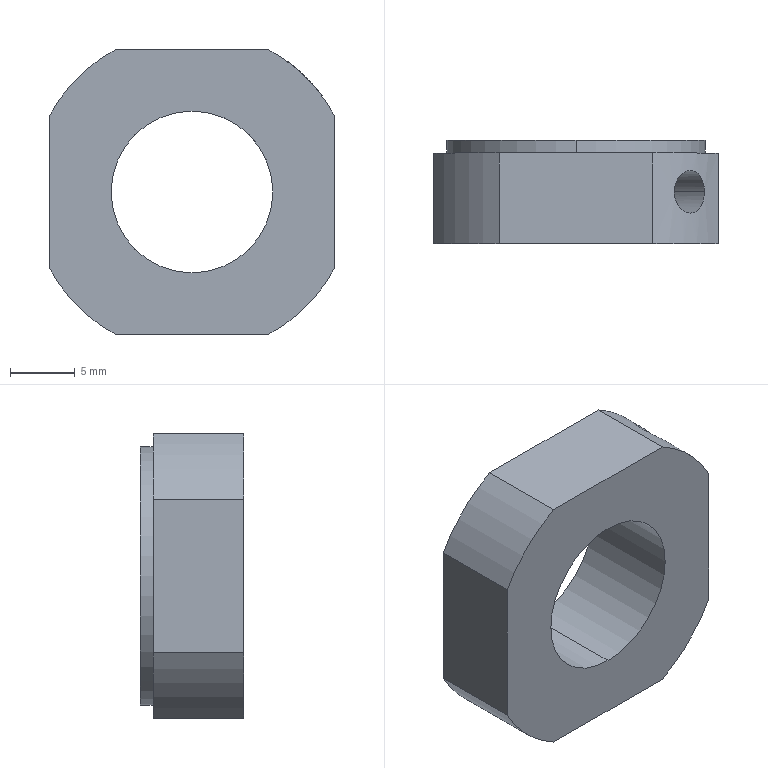Part | STEP file | 1 solid | 17 faces | box 22 x 8 x 22 mm | volume 2378 mm3 | cylinder 10 | plane 7 | commonest cylinder face diameters 25 x4 3.3 x2 12.5 x2 20 x2